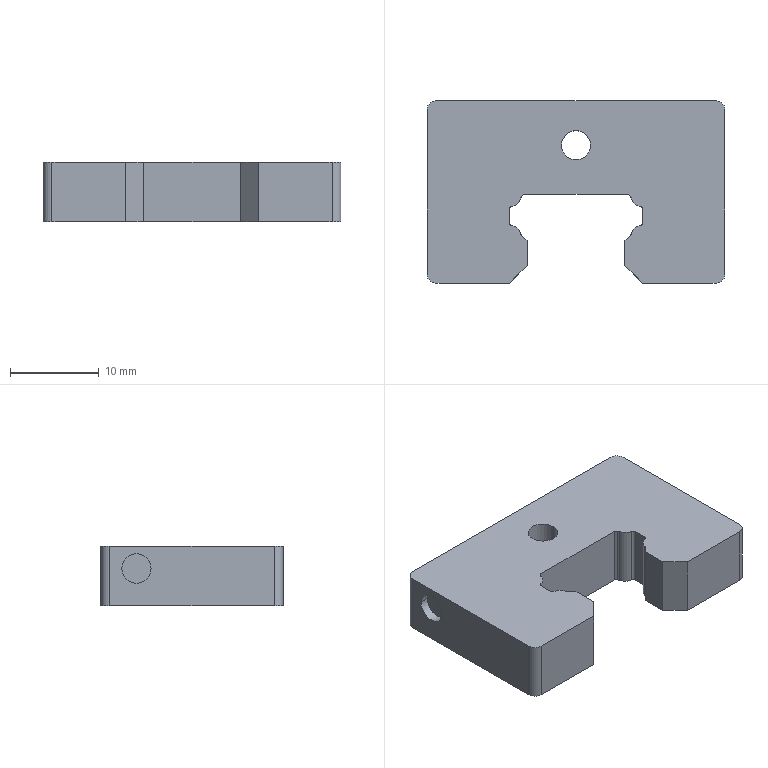Part | SolidWorks | features BaseBody 1 | 1 solid | 42 faces | box 33.5 x 20.5 x 6.7 mm | volume 3669 mm3 | cylinder 22 | plane 20 | commonest cylinder face diameters 0.6 x8 3.3 x6 2 x4 2.6 x4
STEP:
#1=CARTESIAN_POINT('',(1.65,7.95,6.7));
#2=VERTEX_POINT('',#1);
#3=CARTESIAN_POINT('',(-1.65,7.95,6.7));
#4=VERTEX_POINT('',#3);
#5=CARTESIAN_POINT('',(0.,7.95,6.7));
#6=DIRECTION('',(0.,0.,-1.));
#7=DIRECTION('',(-1.,0.,0.));
#8=AXIS2_PLACEMENT_3D('',#5,#6,#7);
#9=CIRCLE('',#8,1.65);
#10=EDGE_CURVE('',#2,#4,#9,.T.);
#11=ORIENTED_EDGE('',*,*,#10,.F.);
#12=CARTESIAN_POINT('',(1.65,7.95,0.));
#13=VERTEX_POINT('',#12);
#14=CARTESIAN_POINT('',(1.65,7.95,6.7));
#15=DIRECTION('',(0.,0.,-1.));
#16=VECTOR('',#15,1000.);
#17=LINE('',#14,#16);
#18=EDGE_CURVE('',#2,#13,#17,.T.);
#19=ORIENTED_EDGE('',*,*,#18,.T.);
#20=CARTESIAN_POINT('',(-1.65,7.95,0.));
#21=VERTEX_POINT('',#20);
#22=CARTESIAN_POINT('',(0.,7.95,0.));
#23=DIRECTION('',(0.,0.,1.));
#24=DIRECTION('',(-1.,0.,0.));
#25=AXIS2_PLACEMENT_3D('',#22,#23,#24);
#26=CIRCLE('',#25,1.65);
#27=EDGE_CURVE('',#21,#13,#26,.T.);
#28=ORIENTED_EDGE('',*,*,#27,.F.);
#29=CARTESIAN_POINT('',(-1.65,7.95,6.7));
#30=DIRECTION('',(0.,0.,-1.));
#31=VECTOR('',#30,1000.);
#32=LINE('',#29,#31);
#33=EDGE_CURVE('',#4,#21,#32,.T.);
#34=ORIENTED_EDGE('',*,*,#33,.F.);
#35=EDGE_LOOP('',(#11,#19,#28,#34));
#36=FACE_OUTER_BOUND('',#35,.T.);
#37=CARTESIAN_POINT('',(0.,7.95,6.7));
#38=DIRECTION('',(0.,0.,-1.));
#39=DIRECTION('',(-1.,0.,0.));
#40=AXIS2_PLACEMENT_3D('',#37,#38,#39);
#41=CYLINDRICAL_SURFACE('',#40,1.65);
#42=ADVANCED_FACE('',(#36),#41,.F.);
#43=CARTESIAN_POINT('',(-15.75,10.6,4.2));
#44=VERTEX_POINT('',#43);
#45=CARTESIAN_POINT('',(-15.75,7.3,4.2));
#46=VERTEX_POINT('',#45);
#47=CARTESIAN_POINT('',(-15.75,8.95,4.2));
#48=DIRECTION('',(-1.,0.,0.));
#49=DIRECTION('',(0.,-1.,0.));
#50=AXIS2_PLACEMENT_3D('',#47,#48,#49);
#51=CIRCLE('',#50,1.65);
#52=EDGE_CURVE('',#44,#46,#51,.T.);
#53=ORIENTED_EDGE('',*,*,#52,.F.);
#54=CARTESIAN_POINT('',(-16.75,10.6,4.2));
#55=VERTEX_POINT('',#54);
#56=CARTESIAN_POINT('',(-15.75,10.6,4.2));
#57=DIRECTION('',(-1.,0.,0.));
#58=VECTOR('',#57,1000.);
#59=LINE('',#56,#58);
#60=EDGE_CURVE('',#44,#55,#59,.T.);
#61=ORIENTED_EDGE('',*,*,#60,.T.);
#62=CARTESIAN_POINT('',(-16.75,7.3,4.2));
#63=VERTEX_POINT('',#62);
#64=CARTESIAN_POINT('',(-16.75,8.95,4.2));
#65=DIRECTION('',(-1.,0.,0.));
#66=DIRECTION('',(0.,-1.,0.));
#67=AXIS2_PLACEMENT_3D('',#64,#65,#66);
#68=CIRCLE('',#67,1.65);
#69=EDGE_CURVE('',#55,#63,#68,.T.);
#70=ORIENTED_EDGE('',*,*,#69,.T.);
#71=CARTESIAN_POINT('',(-15.75,7.3,4.2));
#72=DIRECTION('',(-1.,0.,0.));
#73=VECTOR('',#72,1000.);
#74=LINE('',#71,#73);
#75=EDGE_CURVE('',#46,#63,#74,.T.);
#76=ORIENTED_EDGE('',*,*,#75,.F.);
#77=EDGE_LOOP('',(#53,#61,#70,#76));
#78=FACE_OUTER_BOUND('',#77,.T.);
#79=CARTESIAN_POINT('',(-15.75,8.95,4.2));
#80=DIRECTION('',(-1.,0.,0.));
#81=DIRECTION('',(0.,-1.,0.));
#82=AXIS2_PLACEMENT_3D('',#79,#80,#81);
#83=CYLINDRICAL_SURFACE('',#82,1.65);
#84=ADVANCED_FACE('',(#78),#83,.F.);
#85=CARTESIAN_POINT('',(15.75,7.3,4.2));
#86=VERTEX_POINT('',#85);
#87=CARTESIAN_POINT('',(15.75,10.6,4.2));
#88=VERTEX_POINT('',#87);
#89=CARTESIAN_POINT('',(15.75,8.95,4.2));
#90=DIRECTION('',(1.,0.,0.));
#91=DIRECTION('',(0.,1.,0.));
#92=AXIS2_PLACEMENT_3D('',#89,#90,#91);
#93=CIRCLE('',#92,1.65);
#94=EDGE_CURVE('',#86,#88,#93,.T.);
#95=ORIENTED_EDGE('',*,*,#94,.F.);
#96=CARTESIAN_POINT('',(16.75,7.3,4.2));
#97=VERTEX_POINT('',#96);
#98=CARTESIAN_POINT('',(15.75,7.3,4.2));
#99=DIRECTION('',(1.,0.,0.));
#100=VECTOR('',#99,1000.);
#101=LINE('',#98,#100);
#102=EDGE_CURVE('',#86,#97,#101,.T.);
#103=ORIENTED_EDGE('',*,*,#102,.T.);
#104=CARTESIAN_POINT('',(16.75,10.6,4.2));
#105=VERTEX_POINT('',#104);
#106=CARTESIAN_POINT('',(16.75,8.95,4.2));
#107=DIRECTION('',(1.,0.,0.));
#108=DIRECTION('',(0.,1.,0.));
#109=AXIS2_PLACEMENT_3D('',#106,#107,#108);
#110=CIRCLE('',#109,1.65);
#111=EDGE_CURVE('',#97,#105,#110,.T.);
#112=ORIENTED_EDGE('',*,*,#111,.T.);
#113=CARTESIAN_POINT('',(15.75,10.6,4.2));
#114=DIRECTION('',(1.,0.,0.));
#115=VECTOR('',#114,1000.);
#116=LINE('',#113,#115);
#117=EDGE_CURVE('',#88,#105,#116,.T.);
#118=ORIENTED_EDGE('',*,*,#117,.F.);
#119=EDGE_LOOP('',(#95,#103,#112,#118));
#120=FACE_OUTER_BOUND('',#119,.T.);
#121=CARTESIAN_POINT('',(15.75,8.95,4.2));
#122=DIRECTION('',(1.,0.,0.));
#123=DIRECTION('',(0.,1.,0.));
#124=AXIS2_PLACEMENT_3D('',#121,#122,#123);
#125=CYLINDRICAL_SURFACE('',#124,1.65);
#126=ADVANCED_FACE('',(#120),#125,.F.);
#127=CARTESIAN_POINT('',(7.5,-0.7541,6.7));
#128=VERTEX_POINT('',#127);
#129=CARTESIAN_POINT('',(7.252,-1.049,6.7));
#130=VERTEX_POINT('',#129);
#131=CARTESIAN_POINT('',(7.2,-0.7541,6.7));
#132=DIRECTION('',(0.,0.,-1.));
#133=DIRECTION('',(-1.,0.,0.));
#134=AXIS2_PLACEMENT_3D('',#131,#132,#133);
#135=CIRCLE('',#134,0.3);
#136=EDGE_CURVE('',#128,#130,#135,.T.);
#137=ORIENTED_EDGE('',*,*,#136,.T.);
#138=CARTESIAN_POINT('',(6.216,-2.022,6.7));
#139=VERTEX_POINT('',#138);
#140=CARTESIAN_POINT('',(7.48,-2.329,6.7));
#141=DIRECTION('',(0.,0.,-1.));
#142=DIRECTION('',(-1.,0.,0.));
#143=AXIS2_PLACEMENT_3D('',#140,#141,#142);
#144=CIRCLE('',#143,1.3);
#145=EDGE_CURVE('',#139,#130,#144,.T.);
#146=ORIENTED_EDGE('',*,*,#145,.F.);
#147=CARTESIAN_POINT('',(6.137,-2.163,6.7));
#148=VERTEX_POINT('',#147);
#149=CARTESIAN_POINT('',(5.925,-1.951,6.7));
#150=DIRECTION('',(0.,0.,-1.));
#151=DIRECTION('',(-1.,0.,0.));
#152=AXIS2_PLACEMENT_3D('',#149,#150,#151);
#153=CIRCLE('',#152,0.3);
#154=EDGE_CURVE('',#139,#148,#153,.T.);
#155=ORIENTED_EDGE('',*,*,#154,.T.);
#156=CARTESIAN_POINT('',(5.5,-2.8,6.7));
#157=VERTEX_POINT('',#156);
#158=CARTESIAN_POINT('',(-9.86,-18.16,6.7));
#159=DIRECTION('',(-0.7071,-0.7071,0.));
#160=VECTOR('',#159,1000.);
#161=LINE('',#158,#160);
#162=EDGE_CURVE('',#148,#157,#161,.T.);
#163=ORIENTED_EDGE('',*,*,#162,.T.);
#164=CARTESIAN_POINT('',(5.5,-5.6,6.7));
#165=VERTEX_POINT('',#164);
#166=CARTESIAN_POINT('',(5.5,-28.022,6.7));
#167=DIRECTION('',(0.,-1.,0.));
#168=VECTOR('',#167,1000.);
#169=LINE('',#166,#168);
#170=EDGE_CURVE('',#157,#165,#169,.T.);
#171=ORIENTED_EDGE('',*,*,#170,.T.);
#172=CARTESIAN_POINT('',(7.45,-7.55,6.7));
#173=VERTEX_POINT('',#172);
#174=CARTESIAN_POINT('',(5.5,-5.6,6.7));
#175=DIRECTION('',(0.7071,-0.7071,0.));
#176=VECTOR('',#175,1000.);
#177=LINE('',#174,#176);
#178=EDGE_CURVE('',#165,#173,#177,.T.);
#179=ORIENTED_EDGE('',*,*,#178,.T.);
#180=CARTESIAN_POINT('',(15.75,-7.55,6.7));
#181=VERTEX_POINT('',#180);
#182=CARTESIAN_POINT('',(0.001224,-7.55,6.7));
#183=DIRECTION('',(1.,0.,0.));
#184=VECTOR('',#183,1000.);
#185=LINE('',#182,#184);
#186=EDGE_CURVE('',#173,#181,#185,.T.);
#187=ORIENTED_EDGE('',*,*,#186,.T.);
#188=CARTESIAN_POINT('',(16.75,-6.55,6.7));
#189=VERTEX_POINT('',#188);
#190=CARTESIAN_POINT('',(15.75,-6.55,6.7));
#191=DIRECTION('',(0.,0.,-1.));
#192=DIRECTION('',(-1.,0.,0.));
#193=AXIS2_PLACEMENT_3D('',#190,#191,#192);
#194=CIRCLE('',#193,1.);
#195=EDGE_CURVE('',#189,#181,#194,.T.);
#196=ORIENTED_EDGE('',*,*,#195,.F.);
#197=CARTESIAN_POINT('',(16.75,11.95,6.7));
#198=VERTEX_POINT('',#197);
#199=CARTESIAN_POINT('',(16.75,-28.022,6.7));
#200=DIRECTION('',(0.,1.,0.));
#201=VECTOR('',#200,1000.);
#202=LINE('',#199,#201);
#203=EDGE_CURVE('',#189,#198,#202,.T.);
#204=ORIENTED_EDGE('',*,*,#203,.T.);
#205=CARTESIAN_POINT('',(15.75,12.95,6.7));
#206=VERTEX_POINT('',#205);
#207=CARTESIAN_POINT('',(15.75,11.95,6.7));
#208=DIRECTION('',(0.,0.,-1.));
#209=DIRECTION('',(-1.,0.,0.));
#210=AXIS2_PLACEMENT_3D('',#207,#208,#209);
#211=CIRCLE('',#210,1.);
#212=EDGE_CURVE('',#206,#198,#211,.T.);
#213=ORIENTED_EDGE('',*,*,#212,.F.);
#214=CARTESIAN_POINT('',(-15.75,12.95,6.7));
#215=VERTEX_POINT('',#214);
#216=CARTESIAN_POINT('',(0.001224,12.95,6.7));
#217=DIRECTION('',(-1.,0.,0.));
#218=VECTOR('',#217,1000.);
#219=LINE('',#216,#218);
#220=EDGE_CURVE('',#206,#215,#219,.T.);
#221=ORIENTED_EDGE('',*,*,#220,.T.);
#222=CARTESIAN_POINT('',(-16.75,11.95,6.7));
#223=VERTEX_POINT('',#222);
#224=CARTESIAN_POINT('',(-15.75,11.95,6.7));
#225=DIRECTION('',(0.,0.,-1.));
#226=DIRECTION('',(-1.,0.,0.));
#227=AXIS2_PLACEMENT_3D('',#224,#225,#226);
#228=CIRCLE('',#227,1.);
#229=EDGE_CURVE('',#223,#215,#228,.T.);
#230=ORIENTED_EDGE('',*,*,#229,.F.);
#231=CARTESIAN_POINT('',(-16.75,-6.55,6.7));
#232=VERTEX_POINT('',#231);
#233=CARTESIAN_POINT('',(-16.75,-28.022,6.7));
#234=DIRECTION('',(0.,-1.,0.));
#235=VECTOR('',#234,1000.);
#236=LINE('',#233,#235);
#237=EDGE_CURVE('',#223,#232,#236,.T.);
#238=ORIENTED_EDGE('',*,*,#237,.T.);
#239=CARTESIAN_POINT('',(-15.75,-7.55,6.7));
#240=VERTEX_POINT('',#239);
#241=CARTESIAN_POINT('',(-15.75,-6.55,6.7));
#242=DIRECTION('',(0.,0.,-1.));
#243=DIRECTION('',(-1.,0.,0.));
#244=AXIS2_PLACEMENT_3D('',#241,#242,#243);
#245=CIRCLE('',#244,1.);
#246=EDGE_CURVE('',#240,#232,#245,.T.);
#247=ORIENTED_EDGE('',*,*,#246,.F.);
#248=CARTESIAN_POINT('',(-7.45,-7.55,6.7));
#249=VERTEX_POINT('',#248);
#250=CARTESIAN_POINT('',(0.001224,-7.55,6.7));
#251=DIRECTION('',(1.,0.,0.));
#252=VECTOR('',#251,1000.);
#253=LINE('',#250,#252);
#254=EDGE_CURVE('',#240,#249,#253,.T.);
#255=ORIENTED_EDGE('',*,*,#254,.T.);
#256=CARTESIAN_POINT('',(-5.5,-5.6,6.7));
#257=VERTEX_POINT('',#256);
#258=CARTESIAN_POINT('',(-7.45,-7.55,6.7));
#259=DIRECTION('',(0.7071,0.7071,0.));
#260=VECTOR('',#259,1000.);
#261=LINE('',#258,#260);
#262=EDGE_CURVE('',#249,#257,#261,.T.);
#263=ORIENTED_EDGE('',*,*,#262,.T.);
#264=CARTESIAN_POINT('',(-5.5,-2.8,6.7));
#265=VERTEX_POINT('',#264);
#266=CARTESIAN_POINT('',(-5.5,-28.022,6.7));
#267=DIRECTION('',(0.,1.,0.));
#268=VECTOR('',#267,1000.);
#269=LINE('',#266,#268);
#270=EDGE_CURVE('',#257,#265,#269,.T.);
#271=ORIENTED_EDGE('',*,*,#270,.T.);
#272=CARTESIAN_POINT('',(-6.137,-2.163,6.7));
#273=VERTEX_POINT('',#272);
#274=CARTESIAN_POINT('',(9.862,-18.162,6.7));
#275=DIRECTION('',(-0.7071,0.7071,0.));
#276=VECTOR('',#275,1000.);
#277=LINE('',#274,#276);
#278=EDGE_CURVE('',#265,#273,#277,.T.);
#279=ORIENTED_EDGE('',*,*,#278,.T.);
#280=CARTESIAN_POINT('',(-6.216,-2.022,6.7));
#281=VERTEX_POINT('',#280);
#282=CARTESIAN_POINT('',(-5.925,-1.951,6.7));
#283=DIRECTION('',(0.,0.,-1.));
#284=DIRECTION('',(-1.,0.,0.));
#285=AXIS2_PLACEMENT_3D('',#282,#283,#284);
#286=CIRCLE('',#285,0.3);
#287=EDGE_CURVE('',#273,#281,#286,.T.);
#288=ORIENTED_EDGE('',*,*,#287,.T.);
#289=CARTESIAN_POINT('',(-7.252,-1.049,6.7));
#290=VERTEX_POINT('',#289);
#291=CARTESIAN_POINT('',(-7.479,-2.33,6.7));
#292=DIRECTION('',(0.,0.,-1.));
#293=DIRECTION('',(-1.,0.,0.));
#294=AXIS2_PLACEMENT_3D('',#291,#292,#293);
#295=CIRCLE('',#294,1.3);
#296=EDGE_CURVE('',#290,#281,#295,.T.);
#297=ORIENTED_EDGE('',*,*,#296,.F.);
#298=CARTESIAN_POINT('',(-7.5,-0.7541,6.7));
#299=VERTEX_POINT('',#298);
#300=CARTESIAN_POINT('',(-7.2,-0.7541,6.7));
#301=DIRECTION('',(0.,0.,-1.));
#302=DIRECTION('',(-1.,0.,0.));
#303=AXIS2_PLACEMENT_3D('',#300,#301,#302);
#304=CIRCLE('',#303,0.3);
#305=EDGE_CURVE('',#290,#299,#304,.T.);
#306=ORIENTED_EDGE('',*,*,#305,.T.);
#307=CARTESIAN_POINT('',(-7.5,0.7541,6.7));
#308=VERTEX_POINT('',#307);
#309=CARTESIAN_POINT('',(-7.5,-28.022,6.7));
#310=DIRECTION('',(0.,-1.,0.));
#311=VECTOR('',#310,1000.);
#312=LINE('',#309,#311);
#313=EDGE_CURVE('',#308,#299,#312,.T.);
#314=ORIENTED_EDGE('',*,*,#313,.F.);
#315=CARTESIAN_POINT('',(-7.252,1.049,6.7));
#316=VERTEX_POINT('',#315);
#317=CARTESIAN_POINT('',(-7.2,0.7541,6.7));
#318=DIRECTION('',(0.,0.,-1.));
#319=DIRECTION('',(-1.,0.,0.));
#320=AXIS2_PLACEMENT_3D('',#317,#318,#319);
#321=CIRCLE('',#320,0.3);
#322=EDGE_CURVE('',#308,#316,#321,.T.);
#323=ORIENTED_EDGE('',*,*,#322,.T.);
#324=CARTESIAN_POINT('',(-6.216,2.022,6.7));
#325=VERTEX_POINT('',#324);
#326=CARTESIAN_POINT('',(-7.48,2.33,6.7));
#327=DIRECTION('',(0.,0.,-1.));
#328=DIRECTION('',(-1.,0.,0.));
#329=AXIS2_PLACEMENT_3D('',#326,#327,#328);
#330=CIRCLE('',#329,1.3);
#331=EDGE_CURVE('',#325,#316,#330,.T.);
#332=ORIENTED_EDGE('',*,*,#331,.F.);
#333=CARTESIAN_POINT('',(-6.137,2.163,6.7));
#334=VERTEX_POINT('',#333);
#335=CARTESIAN_POINT('',(-5.925,1.951,6.7));
#336=DIRECTION('',(0.,0.,-1.));
#337=DIRECTION('',(-1.,0.,0.));
#338=AXIS2_PLACEMENT_3D('',#335,#336,#337);
#339=CIRCLE('',#338,0.3);
#340=EDGE_CURVE('',#325,#334,#339,.T.);
#341=ORIENTED_EDGE('',*,*,#340,.T.);
#342=CARTESIAN_POINT('',(-5.85,2.45,6.7));
#343=VERTEX_POINT('',#342);
#344=CARTESIAN_POINT('',(-18.16,-9.86,6.7));
#345=DIRECTION('',(0.7071,0.7071,0.));
#346=VECTOR('',#345,1000.);
#347=LINE('',#344,#346);
#348=EDGE_CURVE('',#334,#343,#347,.T.);
#349=ORIENTED_EDGE('',*,*,#348,.T.);
#350=CARTESIAN_POINT('',(5.85,2.45,6.7));
#351=VERTEX_POINT('',#350);
#352=CARTESIAN_POINT('',(0.001224,2.45,6.7));
#353=DIRECTION('',(1.,0.,0.));
#354=VECTOR('',#353,1000.);
#355=LINE('',#352,#354);
#356=EDGE_CURVE('',#343,#351,#355,.T.);
#357=ORIENTED_EDGE('',*,*,#356,.T.);
#358=CARTESIAN_POINT('',(6.137,2.163,6.7));
#359=VERTEX_POINT('',#358);
#360=CARTESIAN_POINT('',(18.162,-9.862,6.7));
#361=DIRECTION('',(0.7071,-0.7071,0.));
#362=VECTOR('',#361,1000.);
#363=LINE('',#360,#362);
#364=EDGE_CURVE('',#351,#359,#363,.T.);
#365=ORIENTED_EDGE('',*,*,#364,.T.);
#366=CARTESIAN_POINT('',(6.216,2.022,6.7));
#367=VERTEX_POINT('',#366);
#368=CARTESIAN_POINT('',(5.925,1.951,6.7));
#369=DIRECTION('',(0.,0.,-1.));
#370=DIRECTION('',(-1.,0.,0.));
#371=AXIS2_PLACEMENT_3D('',#368,#369,#370);
#372=CIRCLE('',#371,0.3);
#373=EDGE_CURVE('',#359,#367,#372,.T.);
#374=ORIENTED_EDGE('',*,*,#373,.T.);
#375=CARTESIAN_POINT('',(7.252,1.049,6.7));
#376=VERTEX_POINT('',#375);
#377=CARTESIAN_POINT('',(7.479,2.33,6.7));
#378=DIRECTION('',(0.,0.,-1.));
#379=DIRECTION('',(-1.,0.,0.));
#380=AXIS2_PLACEMENT_3D('',#377,#378,#379);
#381=CIRCLE('',#380,1.3);
#382=EDGE_CURVE('',#376,#367,#381,.T.);
#383=ORIENTED_EDGE('',*,*,#382,.F.);
#384=CARTESIAN_POINT('',(7.5,0.7541,6.7));
#385=VERTEX_POINT('',#384);
#386=CARTESIAN_POINT('',(7.2,0.7541,6.7));
#387=DIRECTION('',(0.,0.,-1.));
#388=DIRECTION('',(-1.,0.,0.));
#389=AXIS2_PLACEMENT_3D('',#386,#387,#388);
#390=CIRCLE('',#389,0.3);
#391=EDGE_CURVE('',#376,#385,#390,.T.);
#392=ORIENTED_EDGE('',*,*,#391,.T.);
#393=CARTESIAN_POINT('',(7.5,-28.022,6.7));
#394=DIRECTION('',(0.,1.,0.));
#395=VECTOR('',#394,1000.);
#396=LINE('',#393,#395);
#397=EDGE_CURVE('',#128,#385,#396,.T.);
#398=ORIENTED_EDGE('',*,*,#397,.F.);
#399=EDGE_LOOP('',(#137,#146,#155,#163,#171,#179,#187,#196,#204,#213,#221,#230,#238,#247,#255,#263,#271,#279,#288,#297,#306,#314,#323,#332,#341,#349,#357,#365,#374,#383,#392,#398));
#400=FACE_OUTER_BOUND('',#399,.T.);
#401=CARTESIAN_POINT('',(0.,7.95,6.7));
#402=DIRECTION('',(0.,0.,-1.));
#403=DIRECTION('',(-1.,0.,0.));
#404=AXIS2_PLACEMENT_3D('',#401,#402,#403);
#405=CIRCLE('',#404,1.65);
#406=EDGE_CURVE('',#4,#2,#405,.T.);
#407=ORIENTED_EDGE('',*,*,#406,.T.);
#408=ORIENTED_EDGE('',*,*,#10,.T.);
#409=EDGE_LOOP('',(#407,#408));
#410=FACE_BOUND('',#409,.T.);
#411=CARTESIAN_POINT('',(0.001224,-28.022,6.7));
#412=DIRECTION('',(0.,0.,1.));
#413=DIRECTION('',(1.,0.,0.));
#414=AXIS2_PLACEMENT_3D('',#411,#412,#413);
#415=PLANE('',#414);
#416=ADVANCED_FACE('',(#400,#410),#415,.T.);
#417=ORIENTED_EDGE('',*,*,#356,.F.);
#418=CARTESIAN_POINT('',(-5.85,2.45,0.));
#419=VERTEX_POINT('',#418);
#420=CARTESIAN_POINT('',(-5.85,2.45,6.7));
#421=DIRECTION('',(0.,0.,-1.));
#422=VECTOR('',#421,1000.);
#423=LINE('',#420,#422);
#424=EDGE_CURVE('',#343,#419,#423,.T.);
#425=ORIENTED_EDGE('',*,*,#424,.T.);
#426=CARTESIAN_POINT('',(5.85,2.45,0.));
#427=VERTEX_POINT('',#426);
#428=CARTESIAN_POINT('',(0.001224,2.45,0.));
#429=DIRECTION('',(1.,0.,0.));
#430=VECTOR('',#429,1000.);
#431=LINE('',#428,#430);
#432=EDGE_CURVE('',#419,#427,#431,.T.);
#433=ORIENTED_EDGE('',*,*,#432,.T.);
#434=CARTESIAN_POINT('',(5.85,2.45,6.7));
#435=DIRECTION('',(0.,0.,1.));
#436=VECTOR('',#435,1000.);
#437=LINE('',#434,#436);
#438=EDGE_CURVE('',#427,#351,#437,.T.);
#439=ORIENTED_EDGE('',*,*,#438,.T.);
#440=EDGE_LOOP('',(#417,#425,#433,#439));
#441=FACE_OUTER_BOUND('',#440,.T.);
#442=CARTESIAN_POINT('',(0.001224,2.45,6.7));
#443=DIRECTION('',(0.,-1.,0.));
#444=DIRECTION('',(0.,0.,-1.));
#445=AXIS2_PLACEMENT_3D('',#442,#443,#444);
#446=PLANE('',#445);
#447=ADVANCED_FACE('',(#441),#446,.T.);
#448=CARTESIAN_POINT('',(-5.5,-2.8,0.));
#449=VERTEX_POINT('',#448);
#450=CARTESIAN_POINT('',(-5.5,-2.8,6.7));
#451=DIRECTION('',(0.,0.,-1.));
#452=VECTOR('',#451,1000.);
#453=LINE('',#450,#452);
#454=EDGE_CURVE('',#265,#449,#453,.T.);
#455=ORIENTED_EDGE('',*,*,#454,.F.);
#456=ORIENTED_EDGE('',*,*,#270,.F.);
#457=CARTESIAN_POINT('',(-5.5,-5.6,0.));
#458=VERTEX_POINT('',#457);
#459=CARTESIAN_POINT('',(-5.5,-5.6,6.7));
#460=DIRECTION('',(0.,0.,1.));
#461=VECTOR('',#460,1000.);
#462=LINE('',#459,#461);
#463=EDGE_CURVE('',#458,#257,#462,.T.);
#464=ORIENTED_EDGE('',*,*,#463,.F.);
#465=CARTESIAN_POINT('',(-5.5,-28.022,0.));
#466=DIRECTION('',(0.,-1.,0.));
#467=VECTOR('',#466,1000.);
#468=LINE('',#465,#467);
#469=EDGE_CURVE('',#449,#458,#468,.T.);
#470=ORIENTED_EDGE('',*,*,#469,.F.);
#471=EDGE_LOOP('',(#455,#456,#464,#470));
#472=FACE_OUTER_BOUND('',#471,.T.);
#473=CARTESIAN_POINT('',(-5.5,-28.022,6.7));
#474=DIRECTION('',(-1.,0.,0.));
#475=DIRECTION('',(0.,0.,1.));
#476=AXIS2_PLACEMENT_3D('',#473,#474,#475);
#477=PLANE('',#476);
#478=ADVANCED_FACE('',(#472),#477,.F.);
#479=ORIENTED_EDGE('',*,*,#463,.T.);
#480=ORIENTED_EDGE('',*,*,#262,.F.);
#481=CARTESIAN_POINT('',(-7.45,-7.55,0.));
#482=VERTEX_POINT('',#481);
#483=CARTESIAN_POINT('',(-7.45,-7.55,6.7));
#484=DIRECTION('',(0.,0.,1.));
#485=VECTOR('',#484,1000.);
#486=LINE('',#483,#485);
#487=EDGE_CURVE('',#482,#249,#486,.T.);
#488=ORIENTED_EDGE('',*,*,#487,.F.);
#489=CARTESIAN_POINT('',(-13.96,-14.06,0.));
#490=DIRECTION('',(-0.7071,-0.7071,0.));
#491=VECTOR('',#490,1000.);
#492=LINE('',#489,#491);
#493=EDGE_CURVE('',#458,#482,#492,.T.);
#494=ORIENTED_EDGE('',*,*,#493,.F.);
#495=EDGE_LOOP('',(#479,#480,#488,#494));
#496=FACE_OUTER_BOUND('',#495,.T.);
#497=CARTESIAN_POINT('',(-13.96,-14.06,6.7));
#498=DIRECTION('',(-0.7071,0.7071,0.));
#499=DIRECTION('',(-0.7071,-0.7071,0.));
#500=AXIS2_PLACEMENT_3D('',#497,#498,#499);
#501=PLANE('',#500);
#502=ADVANCED_FACE('',(#496),#501,.F.);
#503=ORIENTED_EDGE('',*,*,#254,.F.);
#504=CARTESIAN_POINT('',(-15.75,-7.55,0.));
#505=VERTEX_POINT('',#504);
#506=CARTESIAN_POINT('',(-15.75,-7.55,6.7));
#507=DIRECTION('',(0.,0.,-1.));
#508=VECTOR('',#507,1000.);
#509=LINE('',#506,#508);
#510=EDGE_CURVE('',#240,#505,#509,.T.);
#511=ORIENTED_EDGE('',*,*,#510,.T.);
#512=CARTESIAN_POINT('',(0.001224,-7.55,0.));
#513=DIRECTION('',(1.,0.,0.));
#514=VECTOR('',#513,1000.);
#515=LINE('',#512,#514);
#516=EDGE_CURVE('',#505,#482,#515,.T.);
#517=ORIENTED_EDGE('',*,*,#516,.T.);
#518=ORIENTED_EDGE('',*,*,#487,.T.);
#519=EDGE_LOOP('',(#503,#511,#517,#518));
#520=FACE_OUTER_BOUND('',#519,.T.);
#521=CARTESIAN_POINT('',(0.001224,-7.55,6.7));
#522=DIRECTION('',(0.,-1.,0.));
#523=DIRECTION('',(1.,0.,0.));
#524=AXIS2_PLACEMENT_3D('',#521,#522,#523);
#525=PLANE('',#524);
#526=ADVANCED_FACE('',(#520),#525,.T.);
#527=CARTESIAN_POINT('',(-16.75,8.95,4.2));
#528=DIRECTION('',(-1.,0.,0.));
#529=DIRECTION('',(0.,-1.,0.));
#530=AXIS2_PLACEMENT_3D('',#527,#528,#529);
#531=CIRCLE('',#530,1.65);
#532=EDGE_CURVE('',#63,#55,#531,.T.);
#533=ORIENTED_EDGE('',*,*,#532,.F.);
#534=ORIENTED_EDGE('',*,*,#69,.F.);
#535=EDGE_LOOP('',(#533,#534));
#536=FACE_BOUND('',#535,.T.);
#537=CARTESIAN_POINT('',(-16.75,-6.55,0.));
#538=VERTEX_POINT('',#537);
#539=CARTESIAN_POINT('',(-16.75,-6.55,6.7));
#540=DIRECTION('',(0.,0.,-1.));
#541=VECTOR('',#540,1000.);
#542=LINE('',#539,#541);
#543=EDGE_CURVE('',#232,#538,#542,.T.);
#544=ORIENTED_EDGE('',*,*,#543,.F.);
#545=ORIENTED_EDGE('',*,*,#237,.F.);
#546=CARTESIAN_POINT('',(-16.75,11.95,0.));
#547=VERTEX_POINT('',#546);
#548=CARTESIAN_POINT('',(-16.75,11.95,6.7));
#549=DIRECTION('',(0.,0.,1.));
#550=VECTOR('',#549,1000.);
#551=LINE('',#548,#550);
#552=EDGE_CURVE('',#547,#223,#551,.T.);
#553=ORIENTED_EDGE('',*,*,#552,.F.);
#554=CARTESIAN_POINT('',(-16.75,-28.022,0.));
#555=DIRECTION('',(0.,1.,0.));
#556=VECTOR('',#555,1000.);
#557=LINE('',#554,#556);
#558=EDGE_CURVE('',#538,#547,#557,.T.);
#559=ORIENTED_EDGE('',*,*,#558,.F.);
#560=EDGE_LOOP('',(#544,#545,#553,#559));
#561=FACE_OUTER_BOUND('',#560,.T.);
#562=CARTESIAN_POINT('',(-16.75,-28.022,6.7));
#563=DIRECTION('',(1.,0.,0.));
#564=DIRECTION('',(0.,1.,0.));
#565=AXIS2_PLACEMENT_3D('',#562,#563,#564);
#566=PLANE('',#565);
#567=ADVANCED_FACE('',(#536,#561),#566,.F.);
#568=ORIENTED_EDGE('',*,*,#220,.F.);
#569=CARTESIAN_POINT('',(15.75,12.95,0.));
#570=VERTEX_POINT('',#569);
#571=CARTESIAN_POINT('',(15.75,12.95,6.7));
#572=DIRECTION('',(0.,0.,-1.));
#573=VECTOR('',#572,1000.);
#574=LINE('',#571,#573);
#575=EDGE_CURVE('',#206,#570,#574,.T.);
#576=ORIENTED_EDGE('',*,*,#575,.T.);
#577=CARTESIAN_POINT('',(-15.75,12.95,0.));
#578=VERTEX_POINT('',#577);
#579=CARTESIAN_POINT('',(0.001224,12.95,0.));
#580=DIRECTION('',(-1.,0.,0.));
#581=VECTOR('',#580,1000.);
#582=LINE('',#579,#581);
#583=EDGE_CURVE('',#570,#578,#582,.T.);
#584=ORIENTED_EDGE('',*,*,#583,.T.);
#585=CARTESIAN_POINT('',(-15.75,12.95,6.7));
#586=DIRECTION('',(0.,0.,1.));
#587=VECTOR('',#586,1000.);
#588=LINE('',#585,#587);
#589=EDGE_CURVE('',#578,#215,#588,.T.);
#590=ORIENTED_EDGE('',*,*,#589,.T.);
#591=EDGE_LOOP('',(#568,#576,#584,#590));
#592=FACE_OUTER_BOUND('',#591,.T.);
#593=CARTESIAN_POINT('',(0.001224,12.95,6.7));
#594=DIRECTION('',(0.,1.,0.));
#595=DIRECTION('',(-1.,0.,0.));
#596=AXIS2_PLACEMENT_3D('',#593,#594,#595);
#597=PLANE('',#596);
#598=ADVANCED_FACE('',(#592),#597,.T.);
#599=CARTESIAN_POINT('',(16.75,11.95,0.));
#600=VERTEX_POINT('',#599);
#601=CARTESIAN_POINT('',(16.75,11.95,6.7));
#602=DIRECTION('',(0.,0.,-1.));
#603=VECTOR('',#602,1000.);
#604=LINE('',#601,#603);
#605=EDGE_CURVE('',#198,#600,#604,.T.);
#606=ORIENTED_EDGE('',*,*,#605,.F.);
#607=ORIENTED_EDGE('',*,*,#203,.F.);
#608=CARTESIAN_POINT('',(16.75,-6.55,0.));
#609=VERTEX_POINT('',#608);
#610=CARTESIAN_POINT('',(16.75,-6.55,6.7));
#611=DIRECTION('',(0.,0.,1.));
#612=VECTOR('',#611,1000.);
#613=LINE('',#610,#612);
#614=EDGE_CURVE('',#609,#189,#613,.T.);
#615=ORIENTED_EDGE('',*,*,#614,.F.);
#616=CARTESIAN_POINT('',(16.75,-28.022,0.));
#617=DIRECTION('',(0.,-1.,0.));
#618=VECTOR('',#617,1000.);
#619=LINE('',#616,#618);
#620=EDGE_CURVE('',#600,#609,#619,.T.);
#621=ORIENTED_EDGE('',*,*,#620,.F.);
#622=EDGE_LOOP('',(#606,#607,#615,#621));
#623=FACE_OUTER_BOUND('',#622,.T.);
#624=CARTESIAN_POINT('',(16.75,8.95,4.2));
#625=DIRECTION('',(1.,0.,0.));
#626=DIRECTION('',(0.,1.,0.));
#627=AXIS2_PLACEMENT_3D('',#624,#625,#626);
#628=CIRCLE('',#627,1.65);
#629=EDGE_CURVE('',#105,#97,#628,.T.);
#630=ORIENTED_EDGE('',*,*,#629,.F.);
#631=ORIENTED_EDGE('',*,*,#111,.F.);
#632=EDGE_LOOP('',(#630,#631));
#633=FACE_BOUND('',#632,.T.);
#634=CARTESIAN_POINT('',(16.75,-28.022,6.7));
#635=DIRECTION('',(-1.,0.,0.));
#636=DIRECTION('',(0.,-1.,0.));
#637=AXIS2_PLACEMENT_3D('',#634,#635,#636);
#638=PLANE('',#637);
#639=ADVANCED_FACE('',(#623,#633),#638,.F.);
#640=CARTESIAN_POINT('',(15.75,-7.55,0.));
#641=VERTEX_POINT('',#640);
#642=CARTESIAN_POINT('',(15.75,-7.55,6.7));
#643=DIRECTION('',(0.,0.,-1.));
#644=VECTOR('',#643,1000.);
#645=LINE('',#642,#644);
#646=EDGE_CURVE('',#181,#641,#645,.T.);
#647=ORIENTED_EDGE('',*,*,#646,.F.);
#648=ORIENTED_EDGE('',*,*,#186,.F.);
#649=CARTESIAN_POINT('',(7.45,-7.55,0.));
#650=VERTEX_POINT('',#649);
#651=CARTESIAN_POINT('',(7.45,-7.55,6.7));
#652=DIRECTION('',(0.,0.,1.));
#653=VECTOR('',#652,1000.);
#654=LINE('',#651,#653);
#655=EDGE_CURVE('',#650,#173,#654,.T.);
#656=ORIENTED_EDGE('',*,*,#655,.F.);
#657=CARTESIAN_POINT('',(0.001224,-7.55,0.));
#658=DIRECTION('',(-1.,0.,0.));
#659=VECTOR('',#658,1000.);
#660=LINE('',#657,#659);
#661=EDGE_CURVE('',#641,#650,#660,.T.);
#662=ORIENTED_EDGE('',*,*,#661,.F.);
#663=EDGE_LOOP('',(#647,#648,#656,#662));
#664=FACE_OUTER_BOUND('',#663,.T.);
#665=CARTESIAN_POINT('',(0.001224,-7.55,6.7));
#666=DIRECTION('',(0.,1.,0.));
#667=DIRECTION('',(-1.,0.,0.));
#668=AXIS2_PLACEMENT_3D('',#665,#666,#667);
#669=PLANE('',#668);
#670=ADVANCED_FACE('',(#664),#669,.F.);
#671=ORIENTED_EDGE('',*,*,#655,.T.);
#672=ORIENTED_EDGE('',*,*,#178,.F.);
#673=CARTESIAN_POINT('',(5.5,-5.6,0.));
#674=VERTEX_POINT('',#673);
#675=CARTESIAN_POINT('',(5.5,-5.6,6.7));
#676=DIRECTION('',(0.,0.,1.));
#677=VECTOR('',#676,1000.);
#678=LINE('',#675,#677);
#679=EDGE_CURVE('',#674,#165,#678,.T.);
#680=ORIENTED_EDGE('',*,*,#679,.F.);
#681=CARTESIAN_POINT('',(13.962,-14.062,0.));
#682=DIRECTION('',(-0.7071,0.7071,0.));
#683=VECTOR('',#682,1000.);
#684=LINE('',#681,#683);
#685=EDGE_CURVE('',#650,#674,#684,.T.);
#686=ORIENTED_EDGE('',*,*,#685,.F.);
#687=EDGE_LOOP('',(#671,#672,#680,#686));
#688=FACE_OUTER_BOUND('',#687,.T.);
#689=CARTESIAN_POINT('',(13.962,-14.062,6.7));
#690=DIRECTION('',(0.7071,0.7071,0.));
#691=DIRECTION('',(-0.7071,0.7071,0.));
#692=AXIS2_PLACEMENT_3D('',#689,#690,#691);
#693=PLANE('',#692);
#694=ADVANCED_FACE('',(#688),#693,.F.);
#695=ORIENTED_EDGE('',*,*,#679,.T.);
#696=ORIENTED_EDGE('',*,*,#170,.F.);
#697=CARTESIAN_POINT('',(5.5,-2.8,0.));
#698=VERTEX_POINT('',#697);
#699=CARTESIAN_POINT('',(5.5,-2.8,6.7));
#700=DIRECTION('',(0.,0.,1.));
#701=VECTOR('',#700,1000.);
#702=LINE('',#699,#701);
#703=EDGE_CURVE('',#698,#157,#702,.T.);
#704=ORIENTED_EDGE('',*,*,#703,.F.);
#705=CARTESIAN_POINT('',(5.5,-28.022,0.));
#706=DIRECTION('',(0.,1.,0.));
#707=VECTOR('',#706,1000.);
#708=LINE('',#705,#707);
#709=EDGE_CURVE('',#674,#698,#708,.T.);
#710=ORIENTED_EDGE('',*,*,#709,.F.);
#711=EDGE_LOOP('',(#695,#696,#704,#710));
#712=FACE_OUTER_BOUND('',#711,.T.);
#713=CARTESIAN_POINT('',(5.5,-28.022,6.7));
#714=DIRECTION('',(1.,0.,0.));
#715=DIRECTION('',(0.,0.,-1.));
#716=AXIS2_PLACEMENT_3D('',#713,#714,#715);
#717=PLANE('',#716);
#718=ADVANCED_FACE('',(#712),#717,.F.);
#719=ORIENTED_EDGE('',*,*,#18,.F.);
#720=ORIENTED_EDGE('',*,*,#406,.F.);
#721=ORIENTED_EDGE('',*,*,#33,.T.);
#722=CARTESIAN_POINT('',(0.,7.95,0.));
#723=DIRECTION('',(0.,0.,1.));
#724=DIRECTION('',(-1.,0.,0.));
#725=AXIS2_PLACEMENT_3D('',#722,#723,#724);
#726=CIRCLE('',#725,1.65);
#727=EDGE_CURVE('',#13,#21,#726,.T.);
#728=ORIENTED_EDGE('',*,*,#727,.F.);
#729=EDGE_LOOP('',(#719,#720,#721,#728));
#730=FACE_OUTER_BOUND('',#729,.T.);
#731=CARTESIAN_POINT('',(0.,7.95,6.7));
#732=DIRECTION('',(0.,0.,-1.));
#733=DIRECTION('',(-1.,0.,0.));
#734=AXIS2_PLACEMENT_3D('',#731,#732,#733);
#735=CYLINDRICAL_SURFACE('',#734,1.65);
#736=ADVANCED_FACE('',(#730),#735,.F.);
#737=ORIENTED_EDGE('',*,*,#424,.F.);
#738=ORIENTED_EDGE('',*,*,#348,.F.);
#739=CARTESIAN_POINT('',(-6.137,2.163,0.));
#740=VERTEX_POINT('',#739);
#741=CARTESIAN_POINT('',(-6.137,2.163,6.7));
#742=DIRECTION('',(0.,0.,1.));
#743=VECTOR('',#742,1000.);
#744=LINE('',#741,#743);
#745=EDGE_CURVE('',#740,#334,#744,.T.);
#746=ORIENTED_EDGE('',*,*,#745,.F.);
#747=CARTESIAN_POINT('',(-18.16,-9.86,0.));
#748=DIRECTION('',(-0.7071,-0.7071,0.));
#749=VECTOR('',#748,1000.);
#750=LINE('',#747,#749);
#751=EDGE_CURVE('',#419,#740,#750,.T.);
#752=ORIENTED_EDGE('',*,*,#751,.F.);
#753=EDGE_LOOP('',(#737,#738,#746,#752));
#754=FACE_OUTER_BOUND('',#753,.T.);
#755=CARTESIAN_POINT('',(-18.16,-9.86,6.7));
#756=DIRECTION('',(-0.7071,0.7071,0.));
#757=DIRECTION('',(-0.7071,-0.7071,0.));
#758=AXIS2_PLACEMENT_3D('',#755,#756,#757);
#759=PLANE('',#758);
#760=ADVANCED_FACE('',(#754),#759,.F.);
#761=CARTESIAN_POINT('',(6.137,2.163,0.));
#762=VERTEX_POINT('',#761);
#763=CARTESIAN_POINT('',(6.137,2.163,6.7));
#764=DIRECTION('',(0.,0.,-1.));
#765=VECTOR('',#764,1000.);
#766=LINE('',#763,#765);
#767=EDGE_CURVE('',#359,#762,#766,.T.);
#768=ORIENTED_EDGE('',*,*,#767,.F.);
#769=ORIENTED_EDGE('',*,*,#364,.F.);
#770=ORIENTED_EDGE('',*,*,#438,.F.);
#771=CARTESIAN_POINT('',(18.162,-9.862,0.));
#772=DIRECTION('',(-0.7071,0.7071,0.));
#773=VECTOR('',#772,1000.);
#774=LINE('',#771,#773);
#775=EDGE_CURVE('',#762,#427,#774,.T.);
#776=ORIENTED_EDGE('',*,*,#775,.F.);
#777=EDGE_LOOP('',(#768,#769,#770,#776));
#778=FACE_OUTER_BOUND('',#777,.T.);
#779=CARTESIAN_POINT('',(18.162,-9.862,6.7));
#780=DIRECTION('',(0.7071,0.7071,0.));
#781=DIRECTION('',(-0.7071,0.7071,0.));
#782=AXIS2_PLACEMENT_3D('',#779,#780,#781);
#783=PLANE('',#782);
#784=ADVANCED_FACE('',(#778),#783,.F.);
#785=CARTESIAN_POINT('',(7.252,-1.049,0.));
#786=VERTEX_POINT('',#785);
#787=CARTESIAN_POINT('',(6.216,-2.022,0.));
#788=VERTEX_POINT('',#787);
#789=CARTESIAN_POINT('',(7.48,-2.329,0.));
#790=DIRECTION('',(0.,0.,1.));
#791=DIRECTION('',(-1.,0.,0.));
#792=AXIS2_PLACEMENT_3D('',#789,#790,#791);
#793=CIRCLE('',#792,1.3);
#794=EDGE_CURVE('',#786,#788,#793,.T.);
#795=ORIENTED_EDGE('',*,*,#794,.F.);
#796=CARTESIAN_POINT('',(7.5,-0.7541,0.));
#797=VERTEX_POINT('',#796);
#798=CARTESIAN_POINT('',(7.2,-0.7541,0.));
#799=DIRECTION('',(0.,0.,1.));
#800=DIRECTION('',(-1.,0.,0.));
#801=AXIS2_PLACEMENT_3D('',#798,#799,#800);
#802=CIRCLE('',#801,0.3);
#803=EDGE_CURVE('',#786,#797,#802,.T.);
#804=ORIENTED_EDGE('',*,*,#803,.T.);
#805=CARTESIAN_POINT('',(7.5,0.7541,0.));
#806=VERTEX_POINT('',#805);
#807=CARTESIAN_POINT('',(7.5,-28.022,0.));
#808=DIRECTION('',(0.,-1.,0.));
#809=VECTOR('',#808,1000.);
#810=LINE('',#807,#809);
#811=EDGE_CURVE('',#806,#797,#810,.T.);
#812=ORIENTED_EDGE('',*,*,#811,.F.);
#813=CARTESIAN_POINT('',(7.252,1.049,0.));
#814=VERTEX_POINT('',#813);
#815=CARTESIAN_POINT('',(7.2,0.7541,0.));
#816=DIRECTION('',(0.,0.,1.));
#817=DIRECTION('',(-1.,0.,0.));
#818=AXIS2_PLACEMENT_3D('',#815,#816,#817);
#819=CIRCLE('',#818,0.3);
#820=EDGE_CURVE('',#806,#814,#819,.T.);
#821=ORIENTED_EDGE('',*,*,#820,.T.);
#822=CARTESIAN_POINT('',(6.216,2.022,0.));
#823=VERTEX_POINT('',#822);
#824=CARTESIAN_POINT('',(7.479,2.33,0.));
#825=DIRECTION('',(0.,0.,1.));
#826=DIRECTION('',(-1.,0.,0.));
#827=AXIS2_PLACEMENT_3D('',#824,#825,#826);
#828=CIRCLE('',#827,1.3);
#829=EDGE_CURVE('',#823,#814,#828,.T.);
#830=ORIENTED_EDGE('',*,*,#829,.F.);
#831=CARTESIAN_POINT('',(5.925,1.951,0.));
#832=DIRECTION('',(0.,0.,-1.));
#833=DIRECTION('',(-1.,0.,0.));
#834=AXIS2_PLACEMENT_3D('',#831,#832,#833);
#835=CIRCLE('',#834,0.3);
#836=EDGE_CURVE('',#762,#823,#835,.T.);
#837=ORIENTED_EDGE('',*,*,#836,.F.);
#838=ORIENTED_EDGE('',*,*,#775,.T.);
#839=ORIENTED_EDGE('',*,*,#432,.F.);
#840=ORIENTED_EDGE('',*,*,#751,.T.);
#841=CARTESIAN_POINT('',(-6.216,2.022,0.));
#842=VERTEX_POINT('',#841);
#843=CARTESIAN_POINT('',(-5.925,1.951,0.));
#844=DIRECTION('',(0.,0.,-1.));
#845=DIRECTION('',(-1.,0.,0.));
#846=AXIS2_PLACEMENT_3D('',#843,#844,#845);
#847=CIRCLE('',#846,0.3);
#848=EDGE_CURVE('',#842,#740,#847,.T.);
#849=ORIENTED_EDGE('',*,*,#848,.F.);
#850=CARTESIAN_POINT('',(-7.252,1.049,0.));
#851=VERTEX_POINT('',#850);
#852=CARTESIAN_POINT('',(-7.48,2.33,0.));
#853=DIRECTION('',(0.,0.,1.));
#854=DIRECTION('',(-1.,0.,0.));
#855=AXIS2_PLACEMENT_3D('',#852,#853,#854);
#856=CIRCLE('',#855,1.3);
#857=EDGE_CURVE('',#851,#842,#856,.T.);
#858=ORIENTED_EDGE('',*,*,#857,.F.);
#859=CARTESIAN_POINT('',(-7.5,0.7541,0.));
#860=VERTEX_POINT('',#859);
#861=CARTESIAN_POINT('',(-7.2,0.7541,0.));
#862=DIRECTION('',(0.,0.,1.));
#863=DIRECTION('',(-1.,0.,0.));
#864=AXIS2_PLACEMENT_3D('',#861,#862,#863);
#865=CIRCLE('',#864,0.3);
#866=EDGE_CURVE('',#851,#860,#865,.T.);
#867=ORIENTED_EDGE('',*,*,#866,.T.);
#868=CARTESIAN_POINT('',(-7.5,-0.7541,0.));
#869=VERTEX_POINT('',#868);
#870=CARTESIAN_POINT('',(-7.5,-28.022,0.));
#871=DIRECTION('',(0.,1.,0.));
#872=VECTOR('',#871,1000.);
#873=LINE('',#870,#872);
#874=EDGE_CURVE('',#869,#860,#873,.T.);
#875=ORIENTED_EDGE('',*,*,#874,.F.);
#876=CARTESIAN_POINT('',(-7.252,-1.049,0.));
#877=VERTEX_POINT('',#876);
#878=CARTESIAN_POINT('',(-7.2,-0.7541,0.));
#879=DIRECTION('',(0.,0.,1.));
#880=DIRECTION('',(-1.,0.,0.));
#881=AXIS2_PLACEMENT_3D('',#878,#879,#880);
#882=CIRCLE('',#881,0.3);
#883=EDGE_CURVE('',#869,#877,#882,.T.);
#884=ORIENTED_EDGE('',*,*,#883,.T.);
#885=CARTESIAN_POINT('',(-6.216,-2.022,0.));
#886=VERTEX_POINT('',#885);
#887=CARTESIAN_POINT('',(-7.479,-2.33,0.));
#888=DIRECTION('',(0.,0.,1.));
#889=DIRECTION('',(-1.,0.,0.));
#890=AXIS2_PLACEMENT_3D('',#887,#888,#889);
#891=CIRCLE('',#890,1.3);
#892=EDGE_CURVE('',#886,#877,#891,.T.);
#893=ORIENTED_EDGE('',*,*,#892,.F.);
#894=CARTESIAN_POINT('',(-6.137,-2.163,0.));
#895=VERTEX_POINT('',#894);
#896=CARTESIAN_POINT('',(-5.925,-1.951,0.));
#897=DIRECTION('',(0.,0.,1.));
#898=DIRECTION('',(-1.,0.,0.));
#899=AXIS2_PLACEMENT_3D('',#896,#897,#898);
#900=CIRCLE('',#899,0.3);
#901=EDGE_CURVE('',#886,#895,#900,.T.);
#902=ORIENTED_EDGE('',*,*,#901,.T.);
#903=CARTESIAN_POINT('',(-5.5,-2.8,0.));
#904=DIRECTION('',(-0.7071,0.7071,0.));
#905=VECTOR('',#904,1000.);
#906=LINE('',#903,#905);
#907=EDGE_CURVE('',#449,#895,#906,.T.);
#908=ORIENTED_EDGE('',*,*,#907,.F.);
#909=ORIENTED_EDGE('',*,*,#469,.T.);
#910=ORIENTED_EDGE('',*,*,#493,.T.);
#911=ORIENTED_EDGE('',*,*,#516,.F.);
#912=CARTESIAN_POINT('',(-15.75,-6.55,0.));
#913=DIRECTION('',(0.,0.,1.));
#914=DIRECTION('',(-1.,0.,0.));
#915=AXIS2_PLACEMENT_3D('',#912,#913,#914);
#916=CIRCLE('',#915,1.);
#917=EDGE_CURVE('',#538,#505,#916,.T.);
#918=ORIENTED_EDGE('',*,*,#917,.F.);
#919=ORIENTED_EDGE('',*,*,#558,.T.);
#920=CARTESIAN_POINT('',(-15.75,11.95,0.));
#921=DIRECTION('',(0.,0.,1.));
#922=DIRECTION('',(-1.,0.,0.));
#923=AXIS2_PLACEMENT_3D('',#920,#921,#922);
#924=CIRCLE('',#923,1.);
#925=EDGE_CURVE('',#578,#547,#924,.T.);
#926=ORIENTED_EDGE('',*,*,#925,.F.);
#927=ORIENTED_EDGE('',*,*,#583,.F.);
#928=CARTESIAN_POINT('',(15.75,11.95,0.));
#929=DIRECTION('',(0.,0.,1.));
#930=DIRECTION('',(-1.,0.,0.));
#931=AXIS2_PLACEMENT_3D('',#928,#929,#930);
#932=CIRCLE('',#931,1.);
#933=EDGE_CURVE('',#600,#570,#932,.T.);
#934=ORIENTED_EDGE('',*,*,#933,.F.);
#935=ORIENTED_EDGE('',*,*,#620,.T.);
#936=CARTESIAN_POINT('',(15.75,-6.55,0.));
#937=DIRECTION('',(0.,0.,1.));
#938=DIRECTION('',(-1.,0.,0.));
#939=AXIS2_PLACEMENT_3D('',#936,#937,#938);
#940=CIRCLE('',#939,1.);
#941=EDGE_CURVE('',#641,#609,#940,.T.);
#942=ORIENTED_EDGE('',*,*,#941,.F.);
#943=ORIENTED_EDGE('',*,*,#661,.T.);
#944=ORIENTED_EDGE('',*,*,#685,.T.);
#945=ORIENTED_EDGE('',*,*,#709,.T.);
#946=CARTESIAN_POINT('',(6.137,-2.163,0.));
#947=VERTEX_POINT('',#946);
#948=CARTESIAN_POINT('',(6.137,-2.163,0.));
#949=DIRECTION('',(-0.7071,-0.7071,0.));
#950=VECTOR('',#949,1000.);
#951=LINE('',#948,#950);
#952=EDGE_CURVE('',#947,#698,#951,.T.);
#953=ORIENTED_EDGE('',*,*,#952,.F.);
#954=CARTESIAN_POINT('',(5.925,-1.951,0.));
#955=DIRECTION('',(0.,0.,1.));
#956=DIRECTION('',(-1.,0.,0.));
#957=AXIS2_PLACEMENT_3D('',#954,#955,#956);
#958=CIRCLE('',#957,0.3);
#959=EDGE_CURVE('',#947,#788,#958,.T.);
#960=ORIENTED_EDGE('',*,*,#959,.T.);
#961=EDGE_LOOP('',(#795,#804,#812,#821,#830,#837,#838,#839,#840,#849,#858,#867,#875,#884,#893,#902,#908,#909,#910,#911,#918,#919,#926,#927,#934,#935,#942,#943,#944,#945,#953,#960));
#962=FACE_OUTER_BOUND('',#961,.T.);
#963=ORIENTED_EDGE('',*,*,#27,.T.);
#964=ORIENTED_EDGE('',*,*,#727,.T.);
#965=EDGE_LOOP('',(#963,#964));
#966=FACE_BOUND('',#965,.T.);
#967=CARTESIAN_POINT('',(0.001224,-28.022,0.));
#968=DIRECTION('',(0.,0.,1.));
#969=DIRECTION('',(1.,0.,0.));
#970=AXIS2_PLACEMENT_3D('',#967,#968,#969);
#971=PLANE('',#970);
#972=ADVANCED_FACE('',(#962,#966),#971,.F.);
#973=CARTESIAN_POINT('',(-6.137,-2.163,6.7));
#974=DIRECTION('',(0.,0.,-1.));
#975=VECTOR('',#974,1000.);
#976=LINE('',#973,#975);
#977=EDGE_CURVE('',#273,#895,#976,.T.);
#978=ORIENTED_EDGE('',*,*,#977,.F.);
#979=ORIENTED_EDGE('',*,*,#278,.F.);
#980=ORIENTED_EDGE('',*,*,#454,.T.);
#981=ORIENTED_EDGE('',*,*,#907,.T.);
#982=EDGE_LOOP('',(#978,#979,#980,#981));
#983=FACE_OUTER_BOUND('',#982,.T.);
#984=CARTESIAN_POINT('',(9.862,-18.162,6.7));
#985=DIRECTION('',(-0.7071,-0.7071,0.));
#986=DIRECTION('',(0.7071,-0.7071,0.));
#987=AXIS2_PLACEMENT_3D('',#984,#985,#986);
#988=PLANE('',#987);
#989=ADVANCED_FACE('',(#983),#988,.F.);
#990=ORIENTED_EDGE('',*,*,#246,.T.);
#991=ORIENTED_EDGE('',*,*,#543,.T.);
#992=ORIENTED_EDGE('',*,*,#917,.T.);
#993=ORIENTED_EDGE('',*,*,#510,.F.);
#994=EDGE_LOOP('',(#990,#991,#992,#993));
#995=FACE_OUTER_BOUND('',#994,.T.);
#996=CARTESIAN_POINT('',(-15.75,-6.55,6.7));
#997=DIRECTION('',(0.,0.,-1.));
#998=DIRECTION('',(-1.,0.,0.));
#999=AXIS2_PLACEMENT_3D('',#996,#997,#998);
#1000=CYLINDRICAL_SURFACE('',#999,1.);
#1001=ADVANCED_FACE('',(#995),#1000,.T.);
#1002=ORIENTED_EDGE('',*,*,#60,.F.);
#1003=CARTESIAN_POINT('',(-15.75,8.95,4.2));
#1004=DIRECTION('',(-1.,0.,0.));
#1005=DIRECTION('',(0.,-1.,0.));
#1006=AXIS2_PLACEMENT_3D('',#1003,#1004,#1005);
#1007=CIRCLE('',#1006,1.65);
#1008=EDGE_CURVE('',#46,#44,#1007,.T.);
#1009=ORIENTED_EDGE('',*,*,#1008,.F.);
#1010=ORIENTED_EDGE('',*,*,#75,.T.);
#1011=ORIENTED_EDGE('',*,*,#532,.T.);
#1012=EDGE_LOOP('',(#1002,#1009,#1010,#1011));
#1013=FACE_OUTER_BOUND('',#1012,.T.);
#1014=CARTESIAN_POINT('',(-15.75,8.95,4.2));
#1015=DIRECTION('',(-1.,0.,0.));
#1016=DIRECTION('',(0.,-1.,0.));
#1017=AXIS2_PLACEMENT_3D('',#1014,#1015,#1016);
#1018=CYLINDRICAL_SURFACE('',#1017,1.65);
#1019=ADVANCED_FACE('',(#1013),#1018,.F.);
#1020=ORIENTED_EDGE('',*,*,#229,.T.);
#1021=ORIENTED_EDGE('',*,*,#589,.F.);
#1022=ORIENTED_EDGE('',*,*,#925,.T.);
#1023=ORIENTED_EDGE('',*,*,#552,.T.);
#1024=EDGE_LOOP('',(#1020,#1021,#1022,#1023));
#1025=FACE_OUTER_BOUND('',#1024,.T.);
#1026=CARTESIAN_POINT('',(-15.75,11.95,6.7));
#1027=DIRECTION('',(0.,0.,-1.));
#1028=DIRECTION('',(-1.,0.,0.));
#1029=AXIS2_PLACEMENT_3D('',#1026,#1027,#1028);
#1030=CYLINDRICAL_SURFACE('',#1029,1.);
#1031=ADVANCED_FACE('',(#1025),#1030,.T.);
#1032=ORIENTED_EDGE('',*,*,#212,.T.);
#1033=ORIENTED_EDGE('',*,*,#605,.T.);
#1034=ORIENTED_EDGE('',*,*,#933,.T.);
#1035=ORIENTED_EDGE('',*,*,#575,.F.);
#1036=EDGE_LOOP('',(#1032,#1033,#1034,#1035));
#1037=FACE_OUTER_BOUND('',#1036,.T.);
#1038=CARTESIAN_POINT('',(15.75,11.95,6.7));
#1039=DIRECTION('',(0.,0.,-1.));
#1040=DIRECTION('',(-1.,0.,0.));
#1041=AXIS2_PLACEMENT_3D('',#1038,#1039,#1040);
#1042=CYLINDRICAL_SURFACE('',#1041,1.);
#1043=ADVANCED_FACE('',(#1037),#1042,.T.);
#1044=ORIENTED_EDGE('',*,*,#195,.T.);
#1045=ORIENTED_EDGE('',*,*,#646,.T.);
#1046=ORIENTED_EDGE('',*,*,#941,.T.);
#1047=ORIENTED_EDGE('',*,*,#614,.T.);
#1048=EDGE_LOOP('',(#1044,#1045,#1046,#1047));
#1049=FACE_OUTER_BOUND('',#1048,.T.);
#1050=CARTESIAN_POINT('',(15.75,-6.55,6.7));
#1051=DIRECTION('',(0.,0.,-1.));
#1052=DIRECTION('',(-1.,0.,0.));
#1053=AXIS2_PLACEMENT_3D('',#1050,#1051,#1052);
#1054=CYLINDRICAL_SURFACE('',#1053,1.);
#1055=ADVANCED_FACE('',(#1049),#1054,.T.);
#1056=ORIENTED_EDGE('',*,*,#102,.F.);
#1057=CARTESIAN_POINT('',(15.75,8.95,4.2));
#1058=DIRECTION('',(1.,0.,0.));
#1059=DIRECTION('',(0.,1.,0.));
#1060=AXIS2_PLACEMENT_3D('',#1057,#1058,#1059);
#1061=CIRCLE('',#1060,1.65);
#1062=EDGE_CURVE('',#88,#86,#1061,.T.);
#1063=ORIENTED_EDGE('',*,*,#1062,.F.);
#1064=ORIENTED_EDGE('',*,*,#117,.T.);
#1065=ORIENTED_EDGE('',*,*,#629,.T.);
#1066=EDGE_LOOP('',(#1056,#1063,#1064,#1065));
#1067=FACE_OUTER_BOUND('',#1066,.T.);
#1068=CARTESIAN_POINT('',(15.75,8.95,4.2));
#1069=DIRECTION('',(1.,0.,0.));
#1070=DIRECTION('',(0.,1.,0.));
#1071=AXIS2_PLACEMENT_3D('',#1068,#1069,#1070);
#1072=CYLINDRICAL_SURFACE('',#1071,1.65);
#1073=ADVANCED_FACE('',(#1067),#1072,.F.);
#1074=ORIENTED_EDGE('',*,*,#703,.T.);
#1075=ORIENTED_EDGE('',*,*,#162,.F.);
#1076=CARTESIAN_POINT('',(6.137,-2.163,6.7));
#1077=DIRECTION('',(0.,0.,1.));
#1078=VECTOR('',#1077,1000.);
#1079=LINE('',#1076,#1078);
#1080=EDGE_CURVE('',#947,#148,#1079,.T.);
#1081=ORIENTED_EDGE('',*,*,#1080,.F.);
#1082=ORIENTED_EDGE('',*,*,#952,.T.);
#1083=EDGE_LOOP('',(#1074,#1075,#1081,#1082));
#1084=FACE_OUTER_BOUND('',#1083,.T.);
#1085=CARTESIAN_POINT('',(-9.86,-18.16,6.7));
#1086=DIRECTION('',(0.7071,-0.7071,0.));
#1087=DIRECTION('',(0.7071,0.7071,0.));
#1088=AXIS2_PLACEMENT_3D('',#1085,#1086,#1087);
#1089=PLANE('',#1088);
#1090=ADVANCED_FACE('',(#1084),#1089,.F.);
#1091=ORIENTED_EDGE('',*,*,#745,.T.);
#1092=ORIENTED_EDGE('',*,*,#340,.F.);
#1093=CARTESIAN_POINT('',(-6.216,2.022,6.7));
#1094=DIRECTION('',(0.,0.,1.));
#1095=VECTOR('',#1094,1000.);
#1096=LINE('',#1093,#1095);
#1097=EDGE_CURVE('',#842,#325,#1096,.T.);
#1098=ORIENTED_EDGE('',*,*,#1097,.F.);
#1099=ORIENTED_EDGE('',*,*,#848,.T.);
#1100=EDGE_LOOP('',(#1091,#1092,#1098,#1099));
#1101=FACE_OUTER_BOUND('',#1100,.T.);
#1102=CARTESIAN_POINT('',(-5.925,1.951,6.7));
#1103=DIRECTION('',(0.,0.,-1.));
#1104=DIRECTION('',(-1.,0.,0.));
#1105=AXIS2_PLACEMENT_3D('',#1102,#1103,#1104);
#1106=CYLINDRICAL_SURFACE('',#1105,0.3);
#1107=ADVANCED_FACE('',(#1101),#1106,.F.);
#1108=CARTESIAN_POINT('',(6.216,2.022,6.7));
#1109=DIRECTION('',(0.,0.,-1.));
#1110=VECTOR('',#1109,1000.);
#1111=LINE('',#1108,#1110);
#1112=EDGE_CURVE('',#367,#823,#1111,.T.);
#1113=ORIENTED_EDGE('',*,*,#1112,.F.);
#1114=ORIENTED_EDGE('',*,*,#373,.F.);
#1115=ORIENTED_EDGE('',*,*,#767,.T.);
#1116=ORIENTED_EDGE('',*,*,#836,.T.);
#1117=EDGE_LOOP('',(#1113,#1114,#1115,#1116));
#1118=FACE_OUTER_BOUND('',#1117,.T.);
#1119=CARTESIAN_POINT('',(5.925,1.951,6.7));
#1120=DIRECTION('',(0.,0.,-1.));
#1121=DIRECTION('',(-1.,0.,0.));
#1122=AXIS2_PLACEMENT_3D('',#1119,#1120,#1121);
#1123=CYLINDRICAL_SURFACE('',#1122,0.3);
#1124=ADVANCED_FACE('',(#1118),#1123,.F.);
#1125=CARTESIAN_POINT('',(-6.216,-2.022,6.7));
#1126=DIRECTION('',(0.,0.,-1.));
#1127=VECTOR('',#1126,1000.);
#1128=LINE('',#1125,#1127);
#1129=EDGE_CURVE('',#281,#886,#1128,.T.);
#1130=ORIENTED_EDGE('',*,*,#1129,.F.);
#1131=ORIENTED_EDGE('',*,*,#287,.F.);
#1132=ORIENTED_EDGE('',*,*,#977,.T.);
#1133=ORIENTED_EDGE('',*,*,#901,.F.);
#1134=EDGE_LOOP('',(#1130,#1131,#1132,#1133));
#1135=FACE_OUTER_BOUND('',#1134,.T.);
#1136=CARTESIAN_POINT('',(-5.925,-1.951,6.7));
#1137=DIRECTION('',(0.,0.,-1.));
#1138=DIRECTION('',(-1.,0.,0.));
#1139=AXIS2_PLACEMENT_3D('',#1136,#1137,#1138);
#1140=CYLINDRICAL_SURFACE('',#1139,0.3);
#1141=ADVANCED_FACE('',(#1135),#1140,.F.);
#1142=ORIENTED_EDGE('',*,*,#1008,.T.);
#1143=ORIENTED_EDGE('',*,*,#52,.T.);
#1144=EDGE_LOOP('',(#1142,#1143));
#1145=FACE_OUTER_BOUND('',#1144,.T.);
#1146=CARTESIAN_POINT('',(-15.75,8.95,4.2));
#1147=DIRECTION('',(-1.,0.,0.));
#1148=DIRECTION('',(0.,-1.,0.));
#1149=AXIS2_PLACEMENT_3D('',#1146,#1147,#1148);
#1150=PLANE('',#1149);
#1151=ADVANCED_FACE('',(#1145),#1150,.T.);
#1152=ORIENTED_EDGE('',*,*,#1062,.T.);
#1153=ORIENTED_EDGE('',*,*,#94,.T.);
#1154=EDGE_LOOP('',(#1152,#1153));
#1155=FACE_OUTER_BOUND('',#1154,.T.);
#1156=CARTESIAN_POINT('',(15.75,8.95,4.2));
#1157=DIRECTION('',(1.,0.,0.));
#1158=DIRECTION('',(0.,1.,0.));
#1159=AXIS2_PLACEMENT_3D('',#1156,#1157,#1158);
#1160=PLANE('',#1159);
#1161=ADVANCED_FACE('',(#1155),#1160,.T.);
#1162=ORIENTED_EDGE('',*,*,#1080,.T.);
#1163=ORIENTED_EDGE('',*,*,#154,.F.);
#1164=CARTESIAN_POINT('',(6.216,-2.022,6.7));
#1165=DIRECTION('',(0.,0.,1.));
#1166=VECTOR('',#1165,1000.);
#1167=LINE('',#1164,#1166);
#1168=EDGE_CURVE('',#788,#139,#1167,.T.);
#1169=ORIENTED_EDGE('',*,*,#1168,.F.);
#1170=ORIENTED_EDGE('',*,*,#959,.F.);
#1171=EDGE_LOOP('',(#1162,#1163,#1169,#1170));
#1172=FACE_OUTER_BOUND('',#1171,.T.);
#1173=CARTESIAN_POINT('',(5.925,-1.951,6.7));
#1174=DIRECTION('',(0.,0.,-1.));
#1175=DIRECTION('',(-1.,0.,0.));
#1176=AXIS2_PLACEMENT_3D('',#1173,#1174,#1175);
#1177=CYLINDRICAL_SURFACE('',#1176,0.3);
#1178=ADVANCED_FACE('',(#1172),#1177,.F.);
#1179=ORIENTED_EDGE('',*,*,#331,.T.);
#1180=CARTESIAN_POINT('',(-7.252,1.049,6.7));
#1181=DIRECTION('',(0.,0.,-1.));
#1182=VECTOR('',#1181,1000.);
#1183=LINE('',#1180,#1182);
#1184=EDGE_CURVE('',#316,#851,#1183,.T.);
#1185=ORIENTED_EDGE('',*,*,#1184,.T.);
#1186=ORIENTED_EDGE('',*,*,#857,.T.);
#1187=ORIENTED_EDGE('',*,*,#1097,.T.);
#1188=EDGE_LOOP('',(#1179,#1185,#1186,#1187));
#1189=FACE_OUTER_BOUND('',#1188,.T.);
#1190=CARTESIAN_POINT('',(-7.48,2.33,6.7));
#1191=DIRECTION('',(0.,0.,-1.));
#1192=DIRECTION('',(-1.,0.,0.));
#1193=AXIS2_PLACEMENT_3D('',#1190,#1191,#1192);
#1194=CYLINDRICAL_SURFACE('',#1193,1.3);
#1195=ADVANCED_FACE('',(#1189),#1194,.T.);
#1196=ORIENTED_EDGE('',*,*,#382,.T.);
#1197=ORIENTED_EDGE('',*,*,#1112,.T.);
#1198=ORIENTED_EDGE('',*,*,#829,.T.);
#1199=CARTESIAN_POINT('',(7.252,1.049,6.7));
#1200=DIRECTION('',(0.,0.,1.));
#1201=VECTOR('',#1200,1000.);
#1202=LINE('',#1199,#1201);
#1203=EDGE_CURVE('',#814,#376,#1202,.T.);
#1204=ORIENTED_EDGE('',*,*,#1203,.T.);
#1205=EDGE_LOOP('',(#1196,#1197,#1198,#1204));
#1206=FACE_OUTER_BOUND('',#1205,.T.);
#1207=CARTESIAN_POINT('',(7.479,2.33,6.7));
#1208=DIRECTION('',(0.,0.,-1.));
#1209=DIRECTION('',(-1.,0.,0.));
#1210=AXIS2_PLACEMENT_3D('',#1207,#1208,#1209);
#1211=CYLINDRICAL_SURFACE('',#1210,1.3);
#1212=ADVANCED_FACE('',(#1206),#1211,.T.);
#1213=ORIENTED_EDGE('',*,*,#296,.T.);
#1214=ORIENTED_EDGE('',*,*,#1129,.T.);
#1215=ORIENTED_EDGE('',*,*,#892,.T.);
#1216=CARTESIAN_POINT('',(-7.252,-1.049,6.7));
#1217=DIRECTION('',(0.,0.,1.));
#1218=VECTOR('',#1217,1000.);
#1219=LINE('',#1216,#1218);
#1220=EDGE_CURVE('',#877,#290,#1219,.T.);
#1221=ORIENTED_EDGE('',*,*,#1220,.T.);
#1222=EDGE_LOOP('',(#1213,#1214,#1215,#1221));
#1223=FACE_OUTER_BOUND('',#1222,.T.);
#1224=CARTESIAN_POINT('',(-7.479,-2.33,6.7));
#1225=DIRECTION('',(0.,0.,-1.));
#1226=DIRECTION('',(-1.,0.,0.));
#1227=AXIS2_PLACEMENT_3D('',#1224,#1225,#1226);
#1228=CYLINDRICAL_SURFACE('',#1227,1.3);
#1229=ADVANCED_FACE('',(#1223),#1228,.T.);
#1230=ORIENTED_EDGE('',*,*,#145,.T.);
#1231=CARTESIAN_POINT('',(7.252,-1.049,6.7));
#1232=DIRECTION('',(0.,0.,-1.));
#1233=VECTOR('',#1232,1000.);
#1234=LINE('',#1231,#1233);
#1235=EDGE_CURVE('',#130,#786,#1234,.T.);
#1236=ORIENTED_EDGE('',*,*,#1235,.T.);
#1237=ORIENTED_EDGE('',*,*,#794,.T.);
#1238=ORIENTED_EDGE('',*,*,#1168,.T.);
#1239=EDGE_LOOP('',(#1230,#1236,#1237,#1238));
#1240=FACE_OUTER_BOUND('',#1239,.T.);
#1241=CARTESIAN_POINT('',(7.48,-2.329,6.7));
#1242=DIRECTION('',(0.,0.,-1.));
#1243=DIRECTION('',(-1.,0.,0.));
#1244=AXIS2_PLACEMENT_3D('',#1241,#1242,#1243);
#1245=CYLINDRICAL_SURFACE('',#1244,1.3);
#1246=ADVANCED_FACE('',(#1240),#1245,.T.);
#1247=ORIENTED_EDGE('',*,*,#1184,.F.);
#1248=ORIENTED_EDGE('',*,*,#322,.F.);
#1249=CARTESIAN_POINT('',(-7.5,0.7541,6.7));
#1250=DIRECTION('',(0.,0.,1.));
#1251=VECTOR('',#1250,1000.);
#1252=LINE('',#1249,#1251);
#1253=EDGE_CURVE('',#860,#308,#1252,.T.);
#1254=ORIENTED_EDGE('',*,*,#1253,.F.);
#1255=ORIENTED_EDGE('',*,*,#866,.F.);
#1256=EDGE_LOOP('',(#1247,#1248,#1254,#1255));
#1257=FACE_OUTER_BOUND('',#1256,.T.);
#1258=CARTESIAN_POINT('',(-7.2,0.7541,6.7));
#1259=DIRECTION('',(0.,0.,-1.));
#1260=DIRECTION('',(-1.,0.,0.));
#1261=AXIS2_PLACEMENT_3D('',#1258,#1259,#1260);
#1262=CYLINDRICAL_SURFACE('',#1261,0.3);
#1263=ADVANCED_FACE('',(#1257),#1262,.F.);
#1264=CARTESIAN_POINT('',(7.5,0.7541,6.7));
#1265=DIRECTION('',(0.,0.,-1.));
#1266=VECTOR('',#1265,1000.);
#1267=LINE('',#1264,#1266);
#1268=EDGE_CURVE('',#385,#806,#1267,.T.);
#1269=ORIENTED_EDGE('',*,*,#1268,.F.);
#1270=ORIENTED_EDGE('',*,*,#391,.F.);
#1271=ORIENTED_EDGE('',*,*,#1203,.F.);
#1272=ORIENTED_EDGE('',*,*,#820,.F.);
#1273=EDGE_LOOP('',(#1269,#1270,#1271,#1272));
#1274=FACE_OUTER_BOUND('',#1273,.T.);
#1275=CARTESIAN_POINT('',(7.2,0.7541,6.7));
#1276=DIRECTION('',(0.,0.,-1.));
#1277=DIRECTION('',(-1.,0.,0.));
#1278=AXIS2_PLACEMENT_3D('',#1275,#1276,#1277);
#1279=CYLINDRICAL_SURFACE('',#1278,0.3);
#1280=ADVANCED_FACE('',(#1274),#1279,.F.);
#1281=CARTESIAN_POINT('',(-7.5,-0.7541,6.7));
#1282=DIRECTION('',(0.,0.,-1.));
#1283=VECTOR('',#1282,1000.);
#1284=LINE('',#1281,#1283);
#1285=EDGE_CURVE('',#299,#869,#1284,.T.);
#1286=ORIENTED_EDGE('',*,*,#1285,.F.);
#1287=ORIENTED_EDGE('',*,*,#305,.F.);
#1288=ORIENTED_EDGE('',*,*,#1220,.F.);
#1289=ORIENTED_EDGE('',*,*,#883,.F.);
#1290=EDGE_LOOP('',(#1286,#1287,#1288,#1289));
#1291=FACE_OUTER_BOUND('',#1290,.T.);
#1292=CARTESIAN_POINT('',(-7.2,-0.7541,6.7));
#1293=DIRECTION('',(0.,0.,-1.));
#1294=DIRECTION('',(-1.,0.,0.));
#1295=AXIS2_PLACEMENT_3D('',#1292,#1293,#1294);
#1296=CYLINDRICAL_SURFACE('',#1295,0.3);
#1297=ADVANCED_FACE('',(#1291),#1296,.F.);
#1298=ORIENTED_EDGE('',*,*,#1235,.F.);
#1299=ORIENTED_EDGE('',*,*,#136,.F.);
#1300=CARTESIAN_POINT('',(7.5,-0.7541,6.7));
#1301=DIRECTION('',(0.,0.,1.));
#1302=VECTOR('',#1301,1000.);
#1303=LINE('',#1300,#1302);
#1304=EDGE_CURVE('',#797,#128,#1303,.T.);
#1305=ORIENTED_EDGE('',*,*,#1304,.F.);
#1306=ORIENTED_EDGE('',*,*,#803,.F.);
#1307=EDGE_LOOP('',(#1298,#1299,#1305,#1306));
#1308=FACE_OUTER_BOUND('',#1307,.T.);
#1309=CARTESIAN_POINT('',(7.2,-0.7541,6.7));
#1310=DIRECTION('',(0.,0.,-1.));
#1311=DIRECTION('',(-1.,0.,0.));
#1312=AXIS2_PLACEMENT_3D('',#1309,#1310,#1311);
#1313=CYLINDRICAL_SURFACE('',#1312,0.3);
#1314=ADVANCED_FACE('',(#1308),#1313,.F.);
#1315=ORIENTED_EDGE('',*,*,#313,.T.);
#1316=ORIENTED_EDGE('',*,*,#1285,.T.);
#1317=ORIENTED_EDGE('',*,*,#874,.T.);
#1318=ORIENTED_EDGE('',*,*,#1253,.T.);
#1319=EDGE_LOOP('',(#1315,#1316,#1317,#1318));
#1320=FACE_OUTER_BOUND('',#1319,.T.);
#1321=CARTESIAN_POINT('',(-7.5,-28.022,6.7));
#1322=DIRECTION('',(1.,0.,0.));
#1323=DIRECTION('',(0.,0.,-1.));
#1324=AXIS2_PLACEMENT_3D('',#1321,#1322,#1323);
#1325=PLANE('',#1324);
#1326=ADVANCED_FACE('',(#1320),#1325,.T.);
#1327=ORIENTED_EDGE('',*,*,#397,.T.);
#1328=ORIENTED_EDGE('',*,*,#1268,.T.);
#1329=ORIENTED_EDGE('',*,*,#811,.T.);
#1330=ORIENTED_EDGE('',*,*,#1304,.T.);
#1331=EDGE_LOOP('',(#1327,#1328,#1329,#1330));
#1332=FACE_OUTER_BOUND('',#1331,.T.);
#1333=CARTESIAN_POINT('',(7.5,-28.022,6.7));
#1334=DIRECTION('',(-1.,0.,0.));
#1335=DIRECTION('',(0.,0.,1.));
#1336=AXIS2_PLACEMENT_3D('',#1333,#1334,#1335);
#1337=PLANE('',#1336);
#1338=ADVANCED_FACE('',(#1332),#1337,.T.);
#1339=CLOSED_SHELL('',(#42,#84,#126,#416,#447,#478,#502,#526,#567,#598,#639,#670,#694,#718,#736,#760,#784,#972,#989,#1001,#1019,#1031,#1043,#1055,#1073,#1090,#1107,#1124,#1141,#1151,#1161,#1178,#1195,#1212,#1229,#1246,#1263,#1280,#1297,#1314,#1326,#1338));
#1340=MANIFOLD_SOLID_BREP('',#1339);
#1341=CARTESIAN_POINT('',(0.,0.,0.));
#1342=DIRECTION('',(0.,0.,1.));
#1343=DIRECTION('',(1.,0.,0.));
#1344=AXIS2_PLACEMENT_3D('',#1341,#1342,#1343);
#1345=(LENGTH_UNIT()NAMED_UNIT(*)SI_UNIT(.MILLI.,.METRE.));
#1346=UNCERTAINTY_MEASURE_WITH_UNIT(LENGTH_MEASURE(0.00001),#1345,'','');
#1347=(NAMED_UNIT(*)PLANE_ANGLE_UNIT()SI_UNIT($,.RADIAN.));
#1348=(NAMED_UNIT(*)SI_UNIT($,.STERADIAN.)SOLID_ANGLE_UNIT());
#1349=(GEOMETRIC_REPRESENTATION_CONTEXT(3)GLOBAL_UNCERTAINTY_ASSIGNED_CONTEXT((#1346))GLOBAL_UNIT_ASSIGNED_CONTEXT((#1345,#1347,#1348))REPRESENTATION_CONTEXT('',''));
#1350=ADVANCED_BREP_SHAPE_REPRESENTATION('',(#1340,#1344),#1349);